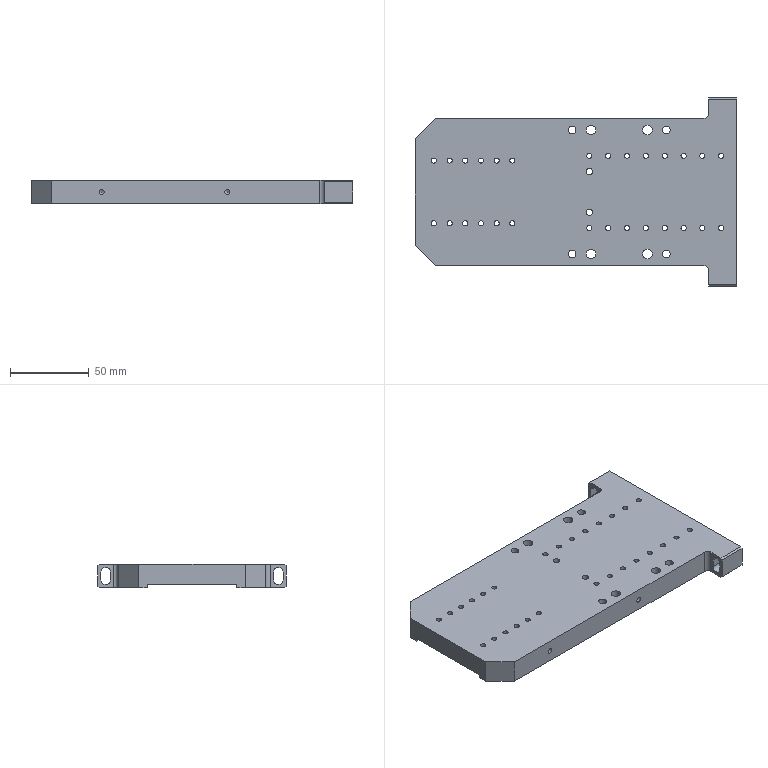Part | 1 solid | 76 faces | box 205 x 120 x 15 mm | volume 261370 mm3 | cylinder 48 | plane 24 | cone 4 | commonest cylinder face diameters 3.3 x32 6 x10 5 x4 4 x2